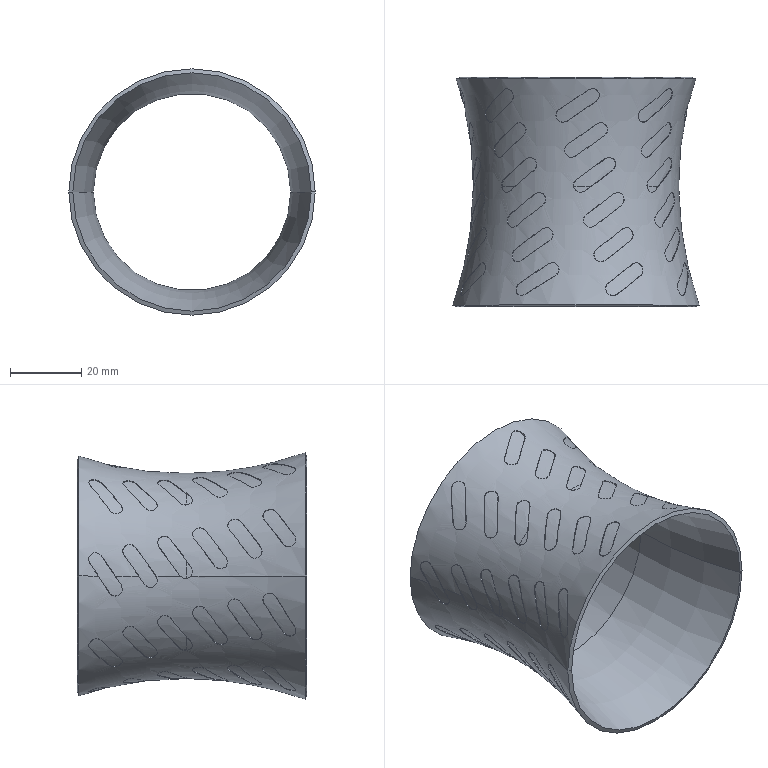Part | SolidWorks | features BaseBody 2, DeleteBody 2, ICE 2, Blend 1, CirPattern 1, Emboss 1, Fillet 1, Helix 1, OffsetRefSurface 1, RefAxis 1, Revolution 1, Sculpt 1, Shell 1, Sweep 1, Thicken 1 | 1 solid | 261 faces | box 69.107 x 64.282 x 69.107 mm | volume 14161 mm3 | spline 192 | torus 65 | cone 4